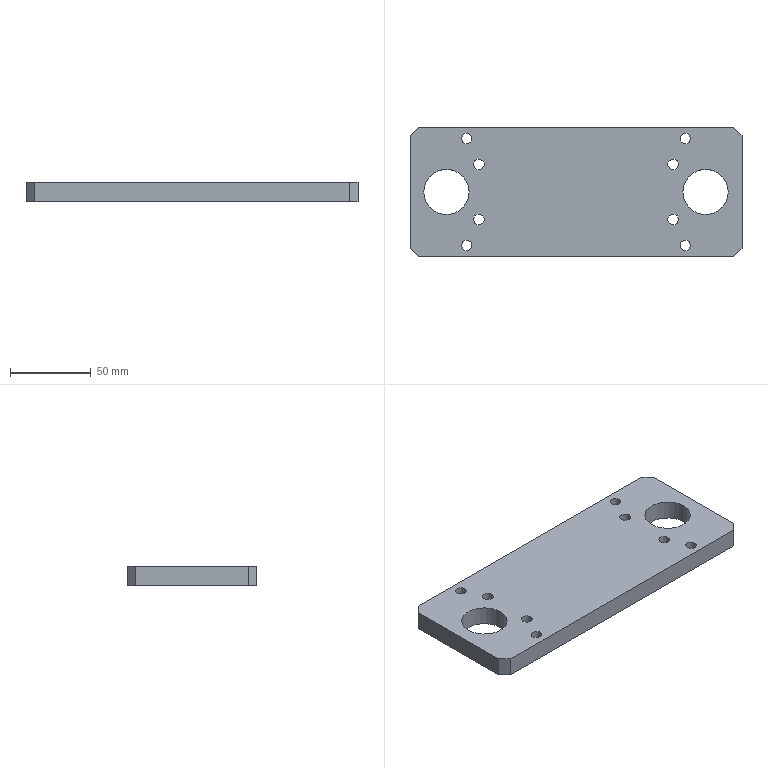Part | NX | features 00 2 | 1 solid | 28 faces | box 205 x 80 x 12 mm | volume 176533 mm3 | cylinder 14 | plane 14 | commonest cylinder face diameters 6.5 x4 6.6 x4 11 x4 28 x2
STEP:
#1=CARTESIAN_POINT('',(54.5,42.,-340.129));
#2=VERTEX_POINT('',#1);
#3=CARTESIAN_POINT('',(60.,42.,-340.129));
#4=DIRECTION('',(0.,0.,1.));
#5=DIRECTION('',(-1.,0.,0.));
#6=AXIS2_PLACEMENT_3D('',#3,#4,#5);
#7=CIRCLE('',#6,5.5);
#8=EDGE_CURVE('',#2,#2,#7,.T.);
#9=ORIENTED_EDGE('',*,*,#8,.F.);
#10=EDGE_LOOP('',(#9));
#11=FACE_BOUND('',#10,.T.);
#12=CARTESIAN_POINT('',(65.5,42.,-333.329));
#13=VERTEX_POINT('',#12);
#14=CARTESIAN_POINT('',(60.,42.,-333.329));
#15=DIRECTION('',(0.,0.,-1.));
#16=DIRECTION('',(1.,0.,0.));
#17=AXIS2_PLACEMENT_3D('',#14,#15,#16);
#18=CIRCLE('',#17,5.5);
#19=EDGE_CURVE('',#13,#13,#18,.T.);
#20=ORIENTED_EDGE('',*,*,#19,.F.);
#21=EDGE_LOOP('',(#20));
#22=FACE_BOUND('',#21,.T.);
#23=CARTESIAN_POINT('',(60.,42.,-340.129));
#24=DIRECTION('',(0.,0.,-1.));
#25=DIRECTION('',(1.,0.,0.));
#26=AXIS2_PLACEMENT_3D('',#23,#24,#25);
#27=CYLINDRICAL_SURFACE('',#26,5.5);
#28=ADVANCED_FACE('',(#11,#22),#27,.F.);
#29=CARTESIAN_POINT('',(56.7,42.,-333.329));
#30=VERTEX_POINT('',#29);
#31=CARTESIAN_POINT('',(60.,42.,-333.329));
#32=DIRECTION('',(0.,0.,1.));
#33=DIRECTION('',(-1.,0.,0.));
#34=AXIS2_PLACEMENT_3D('',#31,#32,#33);
#35=CIRCLE('',#34,3.3);
#36=EDGE_CURVE('',#30,#30,#35,.T.);
#37=ORIENTED_EDGE('',*,*,#36,.T.);
#38=EDGE_LOOP('',(#37));
#39=FACE_BOUND('',#38,.T.);
#40=ORIENTED_EDGE('',*,*,#19,.T.);
#41=EDGE_LOOP('',(#40));
#42=FACE_BOUND('',#41,.T.);
#43=CARTESIAN_POINT('',(56.7,42.,-333.329));
#44=DIRECTION('',(0.,0.,1.));
#45=DIRECTION('',(-1.,0.,0.));
#46=AXIS2_PLACEMENT_3D('',#43,#44,#45);
#47=PLANE('',#46);
#48=ADVANCED_FACE('',(#39,#42),#47,.F.);
#49=CARTESIAN_POINT('',(63.3,42.,-328.129));
#50=VERTEX_POINT('',#49);
#51=CARTESIAN_POINT('',(60.,42.,-328.129));
#52=DIRECTION('',(0.,0.,-1.));
#53=DIRECTION('',(1.,0.,0.));
#54=AXIS2_PLACEMENT_3D('',#51,#52,#53);
#55=CIRCLE('',#54,3.3);
#56=EDGE_CURVE('',#50,#50,#55,.T.);
#57=ORIENTED_EDGE('',*,*,#56,.F.);
#58=EDGE_LOOP('',(#57));
#59=FACE_BOUND('',#58,.T.);
#60=ORIENTED_EDGE('',*,*,#36,.F.);
#61=EDGE_LOOP('',(#60));
#62=FACE_BOUND('',#61,.T.);
#63=CARTESIAN_POINT('',(60.,42.,-340.129));
#64=DIRECTION('',(0.,0.,-1.));
#65=DIRECTION('',(1.,0.,0.));
#66=AXIS2_PLACEMENT_3D('',#63,#64,#65);
#67=CYLINDRICAL_SURFACE('',#66,3.3);
#68=ADVANCED_FACE('',(#59,#62),#67,.F.);
#69=CARTESIAN_POINT('',(65.5,8.,-333.329));
#70=VERTEX_POINT('',#69);
#71=CARTESIAN_POINT('',(60.,8.,-333.329));
#72=DIRECTION('',(0.,0.,-1.));
#73=DIRECTION('',(1.,0.,0.));
#74=AXIS2_PLACEMENT_3D('',#71,#72,#73);
#75=CIRCLE('',#74,5.5);
#76=EDGE_CURVE('',#70,#70,#75,.T.);
#77=ORIENTED_EDGE('',*,*,#76,.F.);
#78=EDGE_LOOP('',(#77));
#79=FACE_BOUND('',#78,.T.);
#80=CARTESIAN_POINT('',(54.5,8.,-340.129));
#81=VERTEX_POINT('',#80);
#82=CARTESIAN_POINT('',(60.,8.,-340.129));
#83=DIRECTION('',(0.,0.,1.));
#84=DIRECTION('',(-1.,0.,0.));
#85=AXIS2_PLACEMENT_3D('',#82,#83,#84);
#86=CIRCLE('',#85,5.5);
#87=EDGE_CURVE('',#81,#81,#86,.T.);
#88=ORIENTED_EDGE('',*,*,#87,.F.);
#89=EDGE_LOOP('',(#88));
#90=FACE_BOUND('',#89,.T.);
#91=CARTESIAN_POINT('',(60.,8.,-340.129));
#92=DIRECTION('',(0.,0.,-1.));
#93=DIRECTION('',(1.,0.,0.));
#94=AXIS2_PLACEMENT_3D('',#91,#92,#93);
#95=CYLINDRICAL_SURFACE('',#94,5.5);
#96=ADVANCED_FACE('',(#79,#90),#95,.F.);
#97=CARTESIAN_POINT('',(56.7,8.,-333.329));
#98=VERTEX_POINT('',#97);
#99=CARTESIAN_POINT('',(60.,8.,-333.329));
#100=DIRECTION('',(0.,0.,1.));
#101=DIRECTION('',(-1.,0.,0.));
#102=AXIS2_PLACEMENT_3D('',#99,#100,#101);
#103=CIRCLE('',#102,3.3);
#104=EDGE_CURVE('',#98,#98,#103,.T.);
#105=ORIENTED_EDGE('',*,*,#104,.T.);
#106=EDGE_LOOP('',(#105));
#107=FACE_BOUND('',#106,.T.);
#108=ORIENTED_EDGE('',*,*,#76,.T.);
#109=EDGE_LOOP('',(#108));
#110=FACE_BOUND('',#109,.T.);
#111=CARTESIAN_POINT('',(56.7,8.,-333.329));
#112=DIRECTION('',(0.,0.,1.));
#113=DIRECTION('',(-1.,0.,0.));
#114=AXIS2_PLACEMENT_3D('',#111,#112,#113);
#115=PLANE('',#114);
#116=ADVANCED_FACE('',(#107,#110),#115,.F.);
#117=ORIENTED_EDGE('',*,*,#104,.F.);
#118=EDGE_LOOP('',(#117));
#119=FACE_BOUND('',#118,.T.);
#120=CARTESIAN_POINT('',(63.3,8.,-328.129));
#121=VERTEX_POINT('',#120);
#122=CARTESIAN_POINT('',(60.,8.,-328.129));
#123=DIRECTION('',(0.,0.,-1.));
#124=DIRECTION('',(1.,0.,0.));
#125=AXIS2_PLACEMENT_3D('',#122,#123,#124);
#126=CIRCLE('',#125,3.3);
#127=EDGE_CURVE('',#121,#121,#126,.T.);
#128=ORIENTED_EDGE('',*,*,#127,.F.);
#129=EDGE_LOOP('',(#128));
#130=FACE_BOUND('',#129,.T.);
#131=CARTESIAN_POINT('',(60.,8.,-340.129));
#132=DIRECTION('',(0.,0.,-1.));
#133=DIRECTION('',(1.,0.,0.));
#134=AXIS2_PLACEMENT_3D('',#131,#132,#133);
#135=CYLINDRICAL_SURFACE('',#134,3.3);
#136=ADVANCED_FACE('',(#119,#130),#135,.F.);
#137=CARTESIAN_POINT('',(-66.,25.,-328.129));
#138=VERTEX_POINT('',#137);
#139=CARTESIAN_POINT('',(-80.,25.,-328.129));
#140=DIRECTION('',(0.,0.,-1.));
#141=DIRECTION('',(1.,0.,0.));
#142=AXIS2_PLACEMENT_3D('',#139,#140,#141);
#143=CIRCLE('',#142,14.);
#144=EDGE_CURVE('',#138,#138,#143,.T.);
#145=ORIENTED_EDGE('',*,*,#144,.F.);
#146=EDGE_LOOP('',(#145));
#147=FACE_BOUND('',#146,.T.);
#148=CARTESIAN_POINT('',(-94.,25.,-340.129));
#149=VERTEX_POINT('',#148);
#150=CARTESIAN_POINT('',(-80.,25.,-340.129));
#151=DIRECTION('',(0.,0.,1.));
#152=DIRECTION('',(-1.,0.,0.));
#153=AXIS2_PLACEMENT_3D('',#150,#151,#152);
#154=CIRCLE('',#153,14.);
#155=EDGE_CURVE('',#149,#149,#154,.T.);
#156=ORIENTED_EDGE('',*,*,#155,.F.);
#157=EDGE_LOOP('',(#156));
#158=FACE_BOUND('',#157,.T.);
#159=CARTESIAN_POINT('',(-80.,25.,-340.129));
#160=DIRECTION('',(0.,0.,1.));
#161=DIRECTION('',(-1.,0.,0.));
#162=AXIS2_PLACEMENT_3D('',#159,#160,#161);
#163=CYLINDRICAL_SURFACE('',#162,14.);
#164=ADVANCED_FACE('',(#147,#158),#163,.F.);
#165=CARTESIAN_POINT('',(94.,25.,-328.129));
#166=VERTEX_POINT('',#165);
#167=CARTESIAN_POINT('',(80.,25.,-328.129));
#168=DIRECTION('',(0.,0.,-1.));
#169=DIRECTION('',(1.,0.,0.));
#170=AXIS2_PLACEMENT_3D('',#167,#168,#169);
#171=CIRCLE('',#170,14.);
#172=EDGE_CURVE('',#166,#166,#171,.T.);
#173=ORIENTED_EDGE('',*,*,#172,.F.);
#174=EDGE_LOOP('',(#173));
#175=FACE_BOUND('',#174,.T.);
#176=CARTESIAN_POINT('',(66.,25.,-340.129));
#177=VERTEX_POINT('',#176);
#178=CARTESIAN_POINT('',(80.,25.,-340.129));
#179=DIRECTION('',(0.,0.,1.));
#180=DIRECTION('',(-1.,0.,0.));
#181=AXIS2_PLACEMENT_3D('',#178,#179,#180);
#182=CIRCLE('',#181,14.);
#183=EDGE_CURVE('',#177,#177,#182,.T.);
#184=ORIENTED_EDGE('',*,*,#183,.F.);
#185=EDGE_LOOP('',(#184));
#186=FACE_BOUND('',#185,.T.);
#187=CARTESIAN_POINT('',(80.,25.,-340.129));
#188=DIRECTION('',(0.,0.,1.));
#189=DIRECTION('',(-1.,0.,0.));
#190=AXIS2_PLACEMENT_3D('',#187,#188,#189);
#191=CYLINDRICAL_SURFACE('',#190,14.);
#192=ADVANCED_FACE('',(#175,#186),#191,.F.);
#193=CARTESIAN_POINT('',(-54.5,42.,-333.329));
#194=VERTEX_POINT('',#193);
#195=CARTESIAN_POINT('',(-60.,42.,-333.329));
#196=DIRECTION('',(0.,0.,-1.));
#197=DIRECTION('',(1.,0.,0.));
#198=AXIS2_PLACEMENT_3D('',#195,#196,#197);
#199=CIRCLE('',#198,5.5);
#200=EDGE_CURVE('',#194,#194,#199,.T.);
#201=ORIENTED_EDGE('',*,*,#200,.F.);
#202=EDGE_LOOP('',(#201));
#203=FACE_BOUND('',#202,.T.);
#204=CARTESIAN_POINT('',(-65.5,42.,-340.129));
#205=VERTEX_POINT('',#204);
#206=CARTESIAN_POINT('',(-60.,42.,-340.129));
#207=DIRECTION('',(0.,0.,1.));
#208=DIRECTION('',(-1.,0.,0.));
#209=AXIS2_PLACEMENT_3D('',#206,#207,#208);
#210=CIRCLE('',#209,5.5);
#211=EDGE_CURVE('',#205,#205,#210,.T.);
#212=ORIENTED_EDGE('',*,*,#211,.F.);
#213=EDGE_LOOP('',(#212));
#214=FACE_BOUND('',#213,.T.);
#215=CARTESIAN_POINT('',(-60.,42.,-340.129));
#216=DIRECTION('',(0.,0.,-1.));
#217=DIRECTION('',(1.,0.,0.));
#218=AXIS2_PLACEMENT_3D('',#215,#216,#217);
#219=CYLINDRICAL_SURFACE('',#218,5.5);
#220=ADVANCED_FACE('',(#203,#214),#219,.F.);
#221=CARTESIAN_POINT('',(-63.3,42.,-333.329));
#222=VERTEX_POINT('',#221);
#223=CARTESIAN_POINT('',(-60.,42.,-333.329));
#224=DIRECTION('',(0.,0.,1.));
#225=DIRECTION('',(-1.,0.,0.));
#226=AXIS2_PLACEMENT_3D('',#223,#224,#225);
#227=CIRCLE('',#226,3.3);
#228=EDGE_CURVE('',#222,#222,#227,.T.);
#229=ORIENTED_EDGE('',*,*,#228,.T.);
#230=EDGE_LOOP('',(#229));
#231=FACE_BOUND('',#230,.T.);
#232=ORIENTED_EDGE('',*,*,#200,.T.);
#233=EDGE_LOOP('',(#232));
#234=FACE_BOUND('',#233,.T.);
#235=CARTESIAN_POINT('',(-63.3,42.,-333.329));
#236=DIRECTION('',(0.,0.,1.));
#237=DIRECTION('',(-1.,0.,0.));
#238=AXIS2_PLACEMENT_3D('',#235,#236,#237);
#239=PLANE('',#238);
#240=ADVANCED_FACE('',(#231,#234),#239,.F.);
#241=CARTESIAN_POINT('',(-56.7,42.,-328.129));
#242=VERTEX_POINT('',#241);
#243=CARTESIAN_POINT('',(-60.,42.,-328.129));
#244=DIRECTION('',(0.,0.,-1.));
#245=DIRECTION('',(1.,0.,0.));
#246=AXIS2_PLACEMENT_3D('',#243,#244,#245);
#247=CIRCLE('',#246,3.3);
#248=EDGE_CURVE('',#242,#242,#247,.T.);
#249=ORIENTED_EDGE('',*,*,#248,.F.);
#250=EDGE_LOOP('',(#249));
#251=FACE_BOUND('',#250,.T.);
#252=ORIENTED_EDGE('',*,*,#228,.F.);
#253=EDGE_LOOP('',(#252));
#254=FACE_BOUND('',#253,.T.);
#255=CARTESIAN_POINT('',(-60.,42.,-340.129));
#256=DIRECTION('',(0.,0.,-1.));
#257=DIRECTION('',(1.,0.,0.));
#258=AXIS2_PLACEMENT_3D('',#255,#256,#257);
#259=CYLINDRICAL_SURFACE('',#258,3.3);
#260=ADVANCED_FACE('',(#251,#254),#259,.F.);
#261=CARTESIAN_POINT('',(-65.5,8.,-340.129));
#262=VERTEX_POINT('',#261);
#263=CARTESIAN_POINT('',(-60.,8.,-340.129));
#264=DIRECTION('',(0.,0.,1.));
#265=DIRECTION('',(-1.,0.,0.));
#266=AXIS2_PLACEMENT_3D('',#263,#264,#265);
#267=CIRCLE('',#266,5.5);
#268=EDGE_CURVE('',#262,#262,#267,.T.);
#269=ORIENTED_EDGE('',*,*,#268,.F.);
#270=EDGE_LOOP('',(#269));
#271=FACE_BOUND('',#270,.T.);
#272=CARTESIAN_POINT('',(-54.5,8.,-333.329));
#273=VERTEX_POINT('',#272);
#274=CARTESIAN_POINT('',(-60.,8.,-333.329));
#275=DIRECTION('',(0.,0.,-1.));
#276=DIRECTION('',(1.,0.,0.));
#277=AXIS2_PLACEMENT_3D('',#274,#275,#276);
#278=CIRCLE('',#277,5.5);
#279=EDGE_CURVE('',#273,#273,#278,.T.);
#280=ORIENTED_EDGE('',*,*,#279,.F.);
#281=EDGE_LOOP('',(#280));
#282=FACE_BOUND('',#281,.T.);
#283=CARTESIAN_POINT('',(-60.,8.,-340.129));
#284=DIRECTION('',(0.,0.,-1.));
#285=DIRECTION('',(1.,0.,0.));
#286=AXIS2_PLACEMENT_3D('',#283,#284,#285);
#287=CYLINDRICAL_SURFACE('',#286,5.5);
#288=ADVANCED_FACE('',(#271,#282),#287,.F.);
#289=CARTESIAN_POINT('',(-63.3,8.,-333.329));
#290=VERTEX_POINT('',#289);
#291=CARTESIAN_POINT('',(-60.,8.,-333.329));
#292=DIRECTION('',(0.,0.,1.));
#293=DIRECTION('',(-1.,0.,0.));
#294=AXIS2_PLACEMENT_3D('',#291,#292,#293);
#295=CIRCLE('',#294,3.3);
#296=EDGE_CURVE('',#290,#290,#295,.T.);
#297=ORIENTED_EDGE('',*,*,#296,.T.);
#298=EDGE_LOOP('',(#297));
#299=FACE_BOUND('',#298,.T.);
#300=ORIENTED_EDGE('',*,*,#279,.T.);
#301=EDGE_LOOP('',(#300));
#302=FACE_BOUND('',#301,.T.);
#303=CARTESIAN_POINT('',(-63.3,8.,-333.329));
#304=DIRECTION('',(0.,0.,1.));
#305=DIRECTION('',(-1.,0.,0.));
#306=AXIS2_PLACEMENT_3D('',#303,#304,#305);
#307=PLANE('',#306);
#308=ADVANCED_FACE('',(#299,#302),#307,.F.);
#309=ORIENTED_EDGE('',*,*,#296,.F.);
#310=EDGE_LOOP('',(#309));
#311=FACE_BOUND('',#310,.T.);
#312=CARTESIAN_POINT('',(-56.7,8.,-328.129));
#313=VERTEX_POINT('',#312);
#314=CARTESIAN_POINT('',(-60.,8.,-328.129));
#315=DIRECTION('',(0.,0.,-1.));
#316=DIRECTION('',(1.,0.,0.));
#317=AXIS2_PLACEMENT_3D('',#314,#315,#316);
#318=CIRCLE('',#317,3.3);
#319=EDGE_CURVE('',#313,#313,#318,.T.);
#320=ORIENTED_EDGE('',*,*,#319,.F.);
#321=EDGE_LOOP('',(#320));
#322=FACE_BOUND('',#321,.T.);
#323=CARTESIAN_POINT('',(-60.,8.,-340.129));
#324=DIRECTION('',(0.,0.,-1.));
#325=DIRECTION('',(1.,0.,0.));
#326=AXIS2_PLACEMENT_3D('',#323,#324,#325);
#327=CYLINDRICAL_SURFACE('',#326,3.3);
#328=ADVANCED_FACE('',(#311,#322),#327,.F.);
#329=CARTESIAN_POINT('',(64.25,58.,-340.129));
#330=VERTEX_POINT('',#329);
#331=CARTESIAN_POINT('',(67.5,58.,-340.129));
#332=DIRECTION('',(0.,0.,1.));
#333=DIRECTION('',(-1.,0.,0.));
#334=AXIS2_PLACEMENT_3D('',#331,#332,#333);
#335=CIRCLE('',#334,3.25);
#336=EDGE_CURVE('',#330,#330,#335,.T.);
#337=ORIENTED_EDGE('',*,*,#336,.F.);
#338=EDGE_LOOP('',(#337));
#339=FACE_BOUND('',#338,.T.);
#340=CARTESIAN_POINT('',(70.75,58.,-328.129));
#341=VERTEX_POINT('',#340);
#342=CARTESIAN_POINT('',(67.5,58.,-328.129));
#343=DIRECTION('',(0.,0.,-1.));
#344=DIRECTION('',(1.,0.,0.));
#345=AXIS2_PLACEMENT_3D('',#342,#343,#344);
#346=CIRCLE('',#345,3.25);
#347=EDGE_CURVE('',#341,#341,#346,.T.);
#348=ORIENTED_EDGE('',*,*,#347,.F.);
#349=EDGE_LOOP('',(#348));
#350=FACE_BOUND('',#349,.T.);
#351=CARTESIAN_POINT('',(67.5,58.,-328.129));
#352=DIRECTION('',(0.,0.,1.));
#353=DIRECTION('',(-1.,0.,0.));
#354=AXIS2_PLACEMENT_3D('',#351,#352,#353);
#355=CYLINDRICAL_SURFACE('',#354,3.25);
#356=ADVANCED_FACE('',(#339,#350),#355,.F.);
#357=CARTESIAN_POINT('',(-64.25,58.,-328.129));
#358=VERTEX_POINT('',#357);
#359=CARTESIAN_POINT('',(-67.5,58.,-328.129));
#360=DIRECTION('',(0.,0.,-1.));
#361=DIRECTION('',(1.,0.,0.));
#362=AXIS2_PLACEMENT_3D('',#359,#360,#361);
#363=CIRCLE('',#362,3.25);
#364=EDGE_CURVE('',#358,#358,#363,.T.);
#365=ORIENTED_EDGE('',*,*,#364,.F.);
#366=EDGE_LOOP('',(#365));
#367=FACE_BOUND('',#366,.T.);
#368=CARTESIAN_POINT('',(-70.75,58.,-340.129));
#369=VERTEX_POINT('',#368);
#370=CARTESIAN_POINT('',(-67.5,58.,-340.129));
#371=DIRECTION('',(0.,0.,1.));
#372=DIRECTION('',(-1.,0.,0.));
#373=AXIS2_PLACEMENT_3D('',#370,#371,#372);
#374=CIRCLE('',#373,3.25);
#375=EDGE_CURVE('',#369,#369,#374,.T.);
#376=ORIENTED_EDGE('',*,*,#375,.F.);
#377=EDGE_LOOP('',(#376));
#378=FACE_BOUND('',#377,.T.);
#379=CARTESIAN_POINT('',(-67.5,58.,-328.129));
#380=DIRECTION('',(0.,0.,1.));
#381=DIRECTION('',(-1.,0.,0.));
#382=AXIS2_PLACEMENT_3D('',#379,#380,#381);
#383=CYLINDRICAL_SURFACE('',#382,3.25);
#384=ADVANCED_FACE('',(#367,#378),#383,.F.);
#385=CARTESIAN_POINT('',(-70.75,-8.,-340.129));
#386=VERTEX_POINT('',#385);
#387=CARTESIAN_POINT('',(-67.5,-8.,-340.129));
#388=DIRECTION('',(0.,0.,1.));
#389=DIRECTION('',(-1.,0.,0.));
#390=AXIS2_PLACEMENT_3D('',#387,#388,#389);
#391=CIRCLE('',#390,3.25);
#392=EDGE_CURVE('',#386,#386,#391,.T.);
#393=ORIENTED_EDGE('',*,*,#392,.F.);
#394=EDGE_LOOP('',(#393));
#395=FACE_BOUND('',#394,.T.);
#396=CARTESIAN_POINT('',(-64.25,-8.,-328.129));
#397=VERTEX_POINT('',#396);
#398=CARTESIAN_POINT('',(-67.5,-8.,-328.129));
#399=DIRECTION('',(0.,0.,-1.));
#400=DIRECTION('',(1.,0.,0.));
#401=AXIS2_PLACEMENT_3D('',#398,#399,#400);
#402=CIRCLE('',#401,3.25);
#403=EDGE_CURVE('',#397,#397,#402,.T.);
#404=ORIENTED_EDGE('',*,*,#403,.F.);
#405=EDGE_LOOP('',(#404));
#406=FACE_BOUND('',#405,.T.);
#407=CARTESIAN_POINT('',(-67.5,-8.,-328.129));
#408=DIRECTION('',(0.,0.,1.));
#409=DIRECTION('',(-1.,0.,0.));
#410=AXIS2_PLACEMENT_3D('',#407,#408,#409);
#411=CYLINDRICAL_SURFACE('',#410,3.25);
#412=ADVANCED_FACE('',(#395,#406),#411,.F.);
#413=CARTESIAN_POINT('',(102.5,60.,-328.129));
#414=VERTEX_POINT('',#413);
#415=CARTESIAN_POINT('',(102.5,60.,-340.129));
#416=VERTEX_POINT('',#415);
#417=CARTESIAN_POINT('',(102.5,60.,-328.129));
#418=DIRECTION('',(0.,0.,-1.));
#419=VECTOR('',#418,1000.);
#420=LINE('',#417,#419);
#421=EDGE_CURVE('',#414,#416,#420,.T.);
#422=ORIENTED_EDGE('',*,*,#421,.T.);
#423=CARTESIAN_POINT('',(97.5,65.,-340.129));
#424=VERTEX_POINT('',#423);
#425=CARTESIAN_POINT('',(97.5,65.,-340.129));
#426=DIRECTION('',(0.7071,-0.7071,0.));
#427=VECTOR('',#426,1000.);
#428=LINE('',#425,#427);
#429=EDGE_CURVE('',#424,#416,#428,.T.);
#430=ORIENTED_EDGE('',*,*,#429,.F.);
#431=CARTESIAN_POINT('',(97.5,65.,-328.129));
#432=VERTEX_POINT('',#431);
#433=CARTESIAN_POINT('',(97.5,65.,-340.129));
#434=DIRECTION('',(0.,0.,1.));
#435=VECTOR('',#434,1000.);
#436=LINE('',#433,#435);
#437=EDGE_CURVE('',#424,#432,#436,.T.);
#438=ORIENTED_EDGE('',*,*,#437,.T.);
#439=CARTESIAN_POINT('',(102.5,60.,-328.129));
#440=DIRECTION('',(-0.7071,0.7071,0.));
#441=VECTOR('',#440,1000.);
#442=LINE('',#439,#441);
#443=EDGE_CURVE('',#414,#432,#442,.T.);
#444=ORIENTED_EDGE('',*,*,#443,.F.);
#445=EDGE_LOOP('',(#422,#430,#438,#444));
#446=FACE_BOUND('',#445,.T.);
#447=CARTESIAN_POINT('',(97.5,65.,-328.129));
#448=DIRECTION('',(-0.7071,-0.7071,0.));
#449=DIRECTION('',(0.,0.,-1.));
#450=AXIS2_PLACEMENT_3D('',#447,#448,#449);
#451=PLANE('',#450);
#452=ADVANCED_FACE('',(#446),#451,.F.);
#453=CARTESIAN_POINT('',(-97.5,65.,-328.129));
#454=VERTEX_POINT('',#453);
#455=CARTESIAN_POINT('',(-97.5,65.,-340.129));
#456=VERTEX_POINT('',#455);
#457=CARTESIAN_POINT('',(-97.5,65.,-328.129));
#458=DIRECTION('',(0.,0.,-1.));
#459=VECTOR('',#458,1000.);
#460=LINE('',#457,#459);
#461=EDGE_CURVE('',#454,#456,#460,.T.);
#462=ORIENTED_EDGE('',*,*,#461,.T.);
#463=CARTESIAN_POINT('',(-102.5,60.,-340.129));
#464=VERTEX_POINT('',#463);
#465=CARTESIAN_POINT('',(-102.5,60.,-340.129));
#466=DIRECTION('',(0.7071,0.7071,0.));
#467=VECTOR('',#466,1000.);
#468=LINE('',#465,#467);
#469=EDGE_CURVE('',#464,#456,#468,.T.);
#470=ORIENTED_EDGE('',*,*,#469,.F.);
#471=CARTESIAN_POINT('',(-102.5,60.,-328.129));
#472=VERTEX_POINT('',#471);
#473=CARTESIAN_POINT('',(-102.5,60.,-340.129));
#474=DIRECTION('',(0.,0.,1.));
#475=VECTOR('',#474,1000.);
#476=LINE('',#473,#475);
#477=EDGE_CURVE('',#464,#472,#476,.T.);
#478=ORIENTED_EDGE('',*,*,#477,.T.);
#479=CARTESIAN_POINT('',(-97.5,65.,-328.129));
#480=DIRECTION('',(-0.7071,-0.7071,0.));
#481=VECTOR('',#480,1000.);
#482=LINE('',#479,#481);
#483=EDGE_CURVE('',#454,#472,#482,.T.);
#484=ORIENTED_EDGE('',*,*,#483,.F.);
#485=EDGE_LOOP('',(#462,#470,#478,#484));
#486=FACE_BOUND('',#485,.T.);
#487=CARTESIAN_POINT('',(-102.5,60.,-328.129));
#488=DIRECTION('',(0.7071,-0.7071,0.));
#489=DIRECTION('',(0.,0.,-1.));
#490=AXIS2_PLACEMENT_3D('',#487,#488,#489);
#491=PLANE('',#490);
#492=ADVANCED_FACE('',(#486),#491,.F.);
#493=ORIENTED_EDGE('',*,*,#477,.F.);
#494=CARTESIAN_POINT('',(-102.5,-10.,-340.129));
#495=VERTEX_POINT('',#494);
#496=CARTESIAN_POINT('',(-102.5,-10.,-340.129));
#497=DIRECTION('',(0.,1.,0.));
#498=VECTOR('',#497,1000.);
#499=LINE('',#496,#498);
#500=EDGE_CURVE('',#495,#464,#499,.T.);
#501=ORIENTED_EDGE('',*,*,#500,.F.);
#502=CARTESIAN_POINT('',(-102.5,-10.,-328.129));
#503=VERTEX_POINT('',#502);
#504=CARTESIAN_POINT('',(-102.5,-10.,-328.129));
#505=DIRECTION('',(0.,0.,-1.));
#506=VECTOR('',#505,1000.);
#507=LINE('',#504,#506);
#508=EDGE_CURVE('',#503,#495,#507,.T.);
#509=ORIENTED_EDGE('',*,*,#508,.F.);
#510=CARTESIAN_POINT('',(-102.5,-10.,-328.129));
#511=DIRECTION('',(0.,1.,0.));
#512=VECTOR('',#511,1000.);
#513=LINE('',#510,#512);
#514=EDGE_CURVE('',#503,#472,#513,.T.);
#515=ORIENTED_EDGE('',*,*,#514,.T.);
#516=EDGE_LOOP('',(#493,#501,#509,#515));
#517=FACE_BOUND('',#516,.T.);
#518=CARTESIAN_POINT('',(-102.5,65.,-328.129));
#519=DIRECTION('',(1.,0.,0.));
#520=DIRECTION('',(0.,0.,1.));
#521=AXIS2_PLACEMENT_3D('',#518,#519,#520);
#522=PLANE('',#521);
#523=ADVANCED_FACE('',(#517),#522,.F.);
#524=ORIENTED_EDGE('',*,*,#508,.T.);
#525=CARTESIAN_POINT('',(-97.5,-15.,-340.129));
#526=VERTEX_POINT('',#525);
#527=CARTESIAN_POINT('',(-97.5,-15.,-340.129));
#528=DIRECTION('',(-0.7071,0.7071,0.));
#529=VECTOR('',#528,1000.);
#530=LINE('',#527,#529);
#531=EDGE_CURVE('',#526,#495,#530,.T.);
#532=ORIENTED_EDGE('',*,*,#531,.F.);
#533=CARTESIAN_POINT('',(-97.5,-15.,-328.129));
#534=VERTEX_POINT('',#533);
#535=CARTESIAN_POINT('',(-97.5,-15.,-340.129));
#536=DIRECTION('',(0.,0.,1.));
#537=VECTOR('',#536,1000.);
#538=LINE('',#535,#537);
#539=EDGE_CURVE('',#526,#534,#538,.T.);
#540=ORIENTED_EDGE('',*,*,#539,.T.);
#541=CARTESIAN_POINT('',(-102.5,-10.,-328.129));
#542=DIRECTION('',(0.7071,-0.7071,0.));
#543=VECTOR('',#542,1000.);
#544=LINE('',#541,#543);
#545=EDGE_CURVE('',#503,#534,#544,.T.);
#546=ORIENTED_EDGE('',*,*,#545,.F.);
#547=EDGE_LOOP('',(#524,#532,#540,#546));
#548=FACE_BOUND('',#547,.T.);
#549=CARTESIAN_POINT('',(-97.5,-15.,-328.129));
#550=DIRECTION('',(0.7071,0.7071,0.));
#551=DIRECTION('',(0.,0.,-1.));
#552=AXIS2_PLACEMENT_3D('',#549,#550,#551);
#553=PLANE('',#552);
#554=ADVANCED_FACE('',(#548),#553,.F.);
#555=CARTESIAN_POINT('',(97.5,-15.,-328.129));
#556=VERTEX_POINT('',#555);
#557=CARTESIAN_POINT('',(97.5,-15.,-340.129));
#558=VERTEX_POINT('',#557);
#559=CARTESIAN_POINT('',(97.5,-15.,-328.129));
#560=DIRECTION('',(0.,0.,-1.));
#561=VECTOR('',#560,1000.);
#562=LINE('',#559,#561);
#563=EDGE_CURVE('',#556,#558,#562,.T.);
#564=ORIENTED_EDGE('',*,*,#563,.F.);
#565=CARTESIAN_POINT('',(97.5,-15.,-328.129));
#566=DIRECTION('',(-1.,0.,0.));
#567=VECTOR('',#566,1000.);
#568=LINE('',#565,#567);
#569=EDGE_CURVE('',#556,#534,#568,.T.);
#570=ORIENTED_EDGE('',*,*,#569,.T.);
#571=ORIENTED_EDGE('',*,*,#539,.F.);
#572=CARTESIAN_POINT('',(97.5,-15.,-340.129));
#573=DIRECTION('',(-1.,0.,0.));
#574=VECTOR('',#573,1000.);
#575=LINE('',#572,#574);
#576=EDGE_CURVE('',#558,#526,#575,.T.);
#577=ORIENTED_EDGE('',*,*,#576,.F.);
#578=EDGE_LOOP('',(#564,#570,#571,#577));
#579=FACE_BOUND('',#578,.T.);
#580=CARTESIAN_POINT('',(-102.5,-15.,-328.129));
#581=DIRECTION('',(0.,1.,0.));
#582=DIRECTION('',(-1.,0.,0.));
#583=AXIS2_PLACEMENT_3D('',#580,#581,#582);
#584=PLANE('',#583);
#585=ADVANCED_FACE('',(#579),#584,.F.);
#586=ORIENTED_EDGE('',*,*,#563,.T.);
#587=CARTESIAN_POINT('',(102.5,-10.,-340.129));
#588=VERTEX_POINT('',#587);
#589=CARTESIAN_POINT('',(102.5,-10.,-340.129));
#590=DIRECTION('',(-0.7071,-0.7071,0.));
#591=VECTOR('',#590,1000.);
#592=LINE('',#589,#591);
#593=EDGE_CURVE('',#588,#558,#592,.T.);
#594=ORIENTED_EDGE('',*,*,#593,.F.);
#595=CARTESIAN_POINT('',(102.5,-10.,-328.129));
#596=VERTEX_POINT('',#595);
#597=CARTESIAN_POINT('',(102.5,-10.,-340.129));
#598=DIRECTION('',(0.,0.,1.));
#599=VECTOR('',#598,1000.);
#600=LINE('',#597,#599);
#601=EDGE_CURVE('',#588,#596,#600,.T.);
#602=ORIENTED_EDGE('',*,*,#601,.T.);
#603=CARTESIAN_POINT('',(97.5,-15.,-328.129));
#604=DIRECTION('',(0.7071,0.7071,0.));
#605=VECTOR('',#604,1000.);
#606=LINE('',#603,#605);
#607=EDGE_CURVE('',#556,#596,#606,.T.);
#608=ORIENTED_EDGE('',*,*,#607,.F.);
#609=EDGE_LOOP('',(#586,#594,#602,#608));
#610=FACE_BOUND('',#609,.T.);
#611=CARTESIAN_POINT('',(102.5,-10.,-328.129));
#612=DIRECTION('',(-0.7071,0.7071,0.));
#613=DIRECTION('',(0.,0.,-1.));
#614=AXIS2_PLACEMENT_3D('',#611,#612,#613);
#615=PLANE('',#614);
#616=ADVANCED_FACE('',(#610),#615,.F.);
#617=ORIENTED_EDGE('',*,*,#421,.F.);
#618=CARTESIAN_POINT('',(102.5,60.,-328.129));
#619=DIRECTION('',(0.,-1.,0.));
#620=VECTOR('',#619,1000.);
#621=LINE('',#618,#620);
#622=EDGE_CURVE('',#414,#596,#621,.T.);
#623=ORIENTED_EDGE('',*,*,#622,.T.);
#624=ORIENTED_EDGE('',*,*,#601,.F.);
#625=CARTESIAN_POINT('',(102.5,60.,-340.129));
#626=DIRECTION('',(0.,-1.,0.));
#627=VECTOR('',#626,1000.);
#628=LINE('',#625,#627);
#629=EDGE_CURVE('',#416,#588,#628,.T.);
#630=ORIENTED_EDGE('',*,*,#629,.F.);
#631=EDGE_LOOP('',(#617,#623,#624,#630));
#632=FACE_BOUND('',#631,.T.);
#633=CARTESIAN_POINT('',(102.5,65.,-328.129));
#634=DIRECTION('',(-1.,0.,0.));
#635=DIRECTION('',(0.,0.,-1.));
#636=AXIS2_PLACEMENT_3D('',#633,#634,#635);
#637=PLANE('',#636);
#638=ADVANCED_FACE('',(#632),#637,.F.);
#639=ORIENTED_EDGE('',*,*,#56,.T.);
#640=EDGE_LOOP('',(#639));
#641=FACE_BOUND('',#640,.T.);
#642=ORIENTED_EDGE('',*,*,#127,.T.);
#643=EDGE_LOOP('',(#642));
#644=FACE_BOUND('',#643,.T.);
#645=ORIENTED_EDGE('',*,*,#144,.T.);
#646=EDGE_LOOP('',(#645));
#647=FACE_BOUND('',#646,.T.);
#648=ORIENTED_EDGE('',*,*,#172,.T.);
#649=EDGE_LOOP('',(#648));
#650=FACE_BOUND('',#649,.T.);
#651=ORIENTED_EDGE('',*,*,#248,.T.);
#652=EDGE_LOOP('',(#651));
#653=FACE_BOUND('',#652,.T.);
#654=ORIENTED_EDGE('',*,*,#319,.T.);
#655=EDGE_LOOP('',(#654));
#656=FACE_BOUND('',#655,.T.);
#657=ORIENTED_EDGE('',*,*,#347,.T.);
#658=EDGE_LOOP('',(#657));
#659=FACE_BOUND('',#658,.T.);
#660=ORIENTED_EDGE('',*,*,#364,.T.);
#661=EDGE_LOOP('',(#660));
#662=FACE_BOUND('',#661,.T.);
#663=ORIENTED_EDGE('',*,*,#403,.T.);
#664=EDGE_LOOP('',(#663));
#665=FACE_BOUND('',#664,.T.);
#666=CARTESIAN_POINT('',(64.25,-8.,-328.129));
#667=VERTEX_POINT('',#666);
#668=CARTESIAN_POINT('',(67.5,-8.,-328.129));
#669=DIRECTION('',(0.,0.,-1.));
#670=DIRECTION('',(-1.,0.,0.));
#671=AXIS2_PLACEMENT_3D('',#668,#669,#670);
#672=CIRCLE('',#671,3.25);
#673=EDGE_CURVE('',#667,#667,#672,.T.);
#674=ORIENTED_EDGE('',*,*,#673,.T.);
#675=EDGE_LOOP('',(#674));
#676=FACE_BOUND('',#675,.T.);
#677=ORIENTED_EDGE('',*,*,#443,.T.);
#678=CARTESIAN_POINT('',(-97.5,65.,-328.129));
#679=DIRECTION('',(1.,0.,0.));
#680=VECTOR('',#679,1000.);
#681=LINE('',#678,#680);
#682=EDGE_CURVE('',#454,#432,#681,.T.);
#683=ORIENTED_EDGE('',*,*,#682,.F.);
#684=ORIENTED_EDGE('',*,*,#483,.T.);
#685=ORIENTED_EDGE('',*,*,#514,.F.);
#686=ORIENTED_EDGE('',*,*,#545,.T.);
#687=ORIENTED_EDGE('',*,*,#569,.F.);
#688=ORIENTED_EDGE('',*,*,#607,.T.);
#689=ORIENTED_EDGE('',*,*,#622,.F.);
#690=EDGE_LOOP('',(#677,#683,#684,#685,#686,#687,#688,#689));
#691=FACE_BOUND('',#690,.T.);
#692=CARTESIAN_POINT('',(0.,25.,-328.129));
#693=DIRECTION('',(0.,0.,1.));
#694=DIRECTION('',(-1.,0.,0.));
#695=AXIS2_PLACEMENT_3D('',#692,#693,#694);
#696=PLANE('',#695);
#697=ADVANCED_FACE('',(#641,#644,#647,#650,#653,#656,#659,#662,#665,#676,#691),#696,.T.);
#698=ORIENTED_EDGE('',*,*,#437,.F.);
#699=CARTESIAN_POINT('',(-97.5,65.,-340.129));
#700=DIRECTION('',(1.,0.,0.));
#701=VECTOR('',#700,1000.);
#702=LINE('',#699,#701);
#703=EDGE_CURVE('',#456,#424,#702,.T.);
#704=ORIENTED_EDGE('',*,*,#703,.F.);
#705=ORIENTED_EDGE('',*,*,#461,.F.);
#706=ORIENTED_EDGE('',*,*,#682,.T.);
#707=EDGE_LOOP('',(#698,#704,#705,#706));
#708=FACE_BOUND('',#707,.T.);
#709=CARTESIAN_POINT('',(-102.5,65.,-328.129));
#710=DIRECTION('',(0.,-1.,0.));
#711=DIRECTION('',(1.,0.,0.));
#712=AXIS2_PLACEMENT_3D('',#709,#710,#711);
#713=PLANE('',#712);
#714=ADVANCED_FACE('',(#708),#713,.F.);
#715=ORIENTED_EDGE('',*,*,#268,.T.);
#716=EDGE_LOOP('',(#715));
#717=FACE_BOUND('',#716,.T.);
#718=ORIENTED_EDGE('',*,*,#211,.T.);
#719=EDGE_LOOP('',(#718));
#720=FACE_BOUND('',#719,.T.);
#721=ORIENTED_EDGE('',*,*,#8,.T.);
#722=EDGE_LOOP('',(#721));
#723=FACE_BOUND('',#722,.T.);
#724=ORIENTED_EDGE('',*,*,#183,.T.);
#725=EDGE_LOOP('',(#724));
#726=FACE_BOUND('',#725,.T.);
#727=ORIENTED_EDGE('',*,*,#155,.T.);
#728=EDGE_LOOP('',(#727));
#729=FACE_BOUND('',#728,.T.);
#730=ORIENTED_EDGE('',*,*,#87,.T.);
#731=EDGE_LOOP('',(#730));
#732=FACE_BOUND('',#731,.T.);
#733=ORIENTED_EDGE('',*,*,#336,.T.);
#734=EDGE_LOOP('',(#733));
#735=FACE_BOUND('',#734,.T.);
#736=ORIENTED_EDGE('',*,*,#375,.T.);
#737=EDGE_LOOP('',(#736));
#738=FACE_BOUND('',#737,.T.);
#739=ORIENTED_EDGE('',*,*,#392,.T.);
#740=EDGE_LOOP('',(#739));
#741=FACE_BOUND('',#740,.T.);
#742=CARTESIAN_POINT('',(70.75,-8.,-340.129));
#743=VERTEX_POINT('',#742);
#744=CARTESIAN_POINT('',(67.5,-8.,-340.129));
#745=DIRECTION('',(0.,0.,1.));
#746=DIRECTION('',(1.,0.,0.));
#747=AXIS2_PLACEMENT_3D('',#744,#745,#746);
#748=CIRCLE('',#747,3.25);
#749=EDGE_CURVE('',#743,#743,#748,.T.);
#750=ORIENTED_EDGE('',*,*,#749,.T.);
#751=EDGE_LOOP('',(#750));
#752=FACE_BOUND('',#751,.T.);
#753=ORIENTED_EDGE('',*,*,#429,.T.);
#754=ORIENTED_EDGE('',*,*,#629,.T.);
#755=ORIENTED_EDGE('',*,*,#593,.T.);
#756=ORIENTED_EDGE('',*,*,#576,.T.);
#757=ORIENTED_EDGE('',*,*,#531,.T.);
#758=ORIENTED_EDGE('',*,*,#500,.T.);
#759=ORIENTED_EDGE('',*,*,#469,.T.);
#760=ORIENTED_EDGE('',*,*,#703,.T.);
#761=EDGE_LOOP('',(#753,#754,#755,#756,#757,#758,#759,#760));
#762=FACE_BOUND('',#761,.T.);
#763=CARTESIAN_POINT('',(0.,25.,-340.129));
#764=DIRECTION('',(0.,0.,1.));
#765=DIRECTION('',(-1.,0.,0.));
#766=AXIS2_PLACEMENT_3D('',#763,#764,#765);
#767=PLANE('',#766);
#768=ADVANCED_FACE('',(#717,#720,#723,#726,#729,#732,#735,#738,#741,#752,#762),#767,.F.);
#769=ORIENTED_EDGE('',*,*,#673,.F.);
#770=EDGE_LOOP('',(#769));
#771=FACE_BOUND('',#770,.T.);
#772=ORIENTED_EDGE('',*,*,#749,.F.);
#773=EDGE_LOOP('',(#772));
#774=FACE_BOUND('',#773,.T.);
#775=CARTESIAN_POINT('',(67.5,-8.,-328.129));
#776=DIRECTION('',(0.,0.,1.));
#777=DIRECTION('',(-1.,0.,0.));
#778=AXIS2_PLACEMENT_3D('',#775,#776,#777);
#779=CYLINDRICAL_SURFACE('',#778,3.25);
#780=ADVANCED_FACE('',(#771,#774),#779,.F.);
#781=CLOSED_SHELL('',(#28,#48,#68,#96,#116,#136,#164,#192,#220,#240,#260,#288,#308,#328,#356,#384,#412,#452,#492,#523,#554,#585,#616,#638,#697,#714,#768,#780));
#782=MANIFOLD_SOLID_BREP('',#781);
#783=(LENGTH_UNIT()NAMED_UNIT(*)SI_UNIT(.MILLI.,.METRE.));
#784=UNCERTAINTY_MEASURE_WITH_UNIT(LENGTH_MEASURE(0.00001),#783,'','');
#785=(NAMED_UNIT(*)PLANE_ANGLE_UNIT()SI_UNIT($,.RADIAN.));
#786=(NAMED_UNIT(*)SI_UNIT($,.STERADIAN.)SOLID_ANGLE_UNIT());
#787=(GEOMETRIC_REPRESENTATION_CONTEXT(3)GLOBAL_UNCERTAINTY_ASSIGNED_CONTEXT((#784))GLOBAL_UNIT_ASSIGNED_CONTEXT((#783,#785,#786))REPRESENTATION_CONTEXT('',''));
#788=ADVANCED_BREP_SHAPE_REPRESENTATION('',(#782),#787);